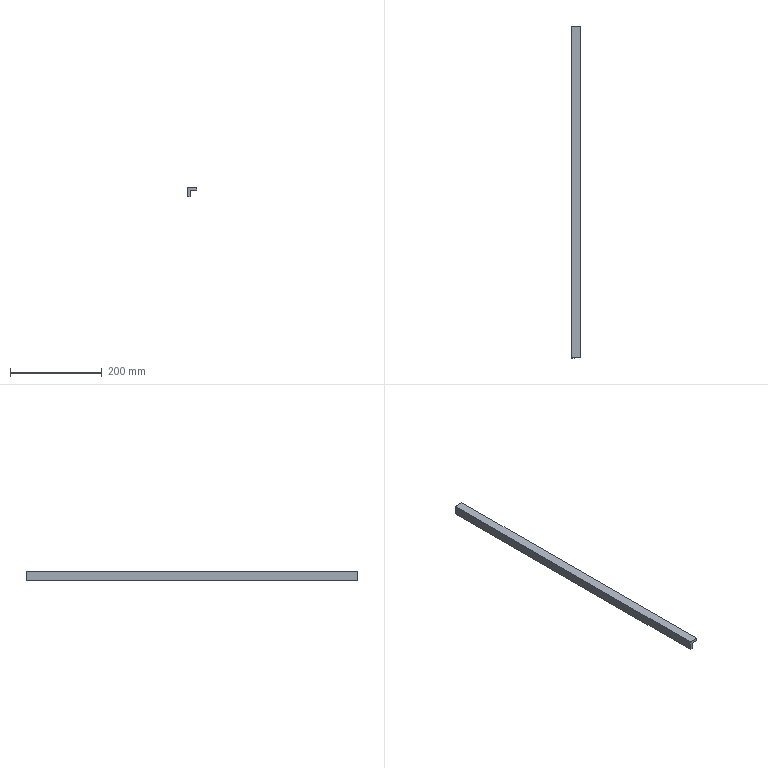Part | NX | 1 solid | 8 faces | box 20 x 724.234 x 20 mm | volume 147744 mm3 | plane 8
STEP:
#1=CARTESIAN_POINT('',(0.,-324.234,0.));
#2=VERTEX_POINT('',#1);
#3=CARTESIAN_POINT('',(20.,-324.234,0.));
#4=VERTEX_POINT('',#3);
#5=CARTESIAN_POINT('',(-266.252,-324.234,0.));
#6=DIRECTION('',(1.,0.,0.));
#7=VECTOR('',#6,1.);
#8=LINE('',#5,#7);
#9=EDGE_CURVE('',#2,#4,#8,.T.);
#10=ORIENTED_EDGE('',*,*,#9,.T.);
#11=CARTESIAN_POINT('',(20.,400.,0.));
#12=VERTEX_POINT('',#11);
#13=CARTESIAN_POINT('',(20.,400.,0.));
#14=DIRECTION('',(0.,-1.,0.));
#15=VECTOR('',#14,1.);
#16=LINE('',#13,#15);
#17=EDGE_CURVE('',#12,#4,#16,.T.);
#18=ORIENTED_EDGE('',*,*,#17,.F.);
#19=CARTESIAN_POINT('',(0.,400.,0.));
#20=VERTEX_POINT('',#19);
#21=CARTESIAN_POINT('',(20.,400.,0.));
#22=DIRECTION('',(1.,0.,0.));
#23=VECTOR('',#22,1.);
#24=LINE('',#21,#23);
#25=EDGE_CURVE('',#20,#12,#24,.T.);
#26=ORIENTED_EDGE('',*,*,#25,.F.);
#27=CARTESIAN_POINT('',(0.,400.,0.));
#28=DIRECTION('',(0.,-1.,0.));
#29=VECTOR('',#28,1.);
#30=LINE('',#27,#29);
#31=EDGE_CURVE('',#20,#2,#30,.T.);
#32=ORIENTED_EDGE('',*,*,#31,.T.);
#33=EDGE_LOOP('',(#10,#18,#26,#32));
#34=FACE_OUTER_BOUND('',#33,.T.);
#35=CARTESIAN_POINT('',(20.,400.,0.));
#36=DIRECTION('',(0.,0.,-1.));
#37=DIRECTION('',(-1.,0.,0.));
#38=AXIS2_PLACEMENT_3D('',#35,#36,#37);
#39=PLANE('',#38);
#40=ADVANCED_FACE('',(#34),#39,.F.);
#41=CARTESIAN_POINT('',(20.,-324.234,-6.));
#42=VERTEX_POINT('',#41);
#43=CARTESIAN_POINT('',(20.,-324.234,-229.311));
#44=DIRECTION('',(0.,0.,-1.));
#45=VECTOR('',#44,1.);
#46=LINE('',#43,#45);
#47=EDGE_CURVE('',#4,#42,#46,.T.);
#48=ORIENTED_EDGE('',*,*,#47,.T.);
#49=CARTESIAN_POINT('',(20.,400.,-6.));
#50=VERTEX_POINT('',#49);
#51=CARTESIAN_POINT('',(20.,400.,-6.));
#52=DIRECTION('',(0.,-1.,0.));
#53=VECTOR('',#52,1.);
#54=LINE('',#51,#53);
#55=EDGE_CURVE('',#50,#42,#54,.T.);
#56=ORIENTED_EDGE('',*,*,#55,.F.);
#57=CARTESIAN_POINT('',(20.,400.,-6.));
#58=DIRECTION('',(0.,0.,-1.));
#59=VECTOR('',#58,1.);
#60=LINE('',#57,#59);
#61=EDGE_CURVE('',#12,#50,#60,.T.);
#62=ORIENTED_EDGE('',*,*,#61,.F.);
#63=ORIENTED_EDGE('',*,*,#17,.T.);
#64=EDGE_LOOP('',(#48,#56,#62,#63));
#65=FACE_OUTER_BOUND('',#64,.T.);
#66=CARTESIAN_POINT('',(20.,400.,-6.));
#67=DIRECTION('',(-1.,0.,0.));
#68=DIRECTION('',(0.,0.,1.));
#69=AXIS2_PLACEMENT_3D('',#66,#67,#68);
#70=PLANE('',#69);
#71=ADVANCED_FACE('',(#65),#70,.F.);
#72=CARTESIAN_POINT('',(6.,-324.234,-6.));
#73=VERTEX_POINT('',#72);
#74=CARTESIAN_POINT('',(-266.252,-324.234,-6.));
#75=DIRECTION('',(-1.,0.,0.));
#76=VECTOR('',#75,1.);
#77=LINE('',#74,#76);
#78=EDGE_CURVE('',#42,#73,#77,.T.);
#79=ORIENTED_EDGE('',*,*,#78,.T.);
#80=CARTESIAN_POINT('',(6.,400.,-6.));
#81=VERTEX_POINT('',#80);
#82=CARTESIAN_POINT('',(6.,400.,-6.));
#83=DIRECTION('',(0.,-1.,0.));
#84=VECTOR('',#83,1.);
#85=LINE('',#82,#84);
#86=EDGE_CURVE('',#81,#73,#85,.T.);
#87=ORIENTED_EDGE('',*,*,#86,.F.);
#88=CARTESIAN_POINT('',(6.,400.,-6.));
#89=DIRECTION('',(-1.,0.,0.));
#90=VECTOR('',#89,1.);
#91=LINE('',#88,#90);
#92=EDGE_CURVE('',#50,#81,#91,.T.);
#93=ORIENTED_EDGE('',*,*,#92,.F.);
#94=ORIENTED_EDGE('',*,*,#55,.T.);
#95=EDGE_LOOP('',(#79,#87,#93,#94));
#96=FACE_OUTER_BOUND('',#95,.T.);
#97=CARTESIAN_POINT('',(6.,400.,-6.));
#98=DIRECTION('',(0.,0.,1.));
#99=DIRECTION('',(1.,0.,0.));
#100=AXIS2_PLACEMENT_3D('',#97,#98,#99);
#101=PLANE('',#100);
#102=ADVANCED_FACE('',(#96),#101,.F.);
#103=CARTESIAN_POINT('',(6.,-324.234,-20.));
#104=VERTEX_POINT('',#103);
#105=CARTESIAN_POINT('',(6.,-324.234,-229.311));
#106=DIRECTION('',(0.,0.,-1.));
#107=VECTOR('',#106,1.);
#108=LINE('',#105,#107);
#109=EDGE_CURVE('',#73,#104,#108,.T.);
#110=ORIENTED_EDGE('',*,*,#109,.T.);
#111=CARTESIAN_POINT('',(6.,400.,-20.));
#112=VERTEX_POINT('',#111);
#113=CARTESIAN_POINT('',(6.,400.,-20.));
#114=DIRECTION('',(0.,-1.,0.));
#115=VECTOR('',#114,1.);
#116=LINE('',#113,#115);
#117=EDGE_CURVE('',#112,#104,#116,.T.);
#118=ORIENTED_EDGE('',*,*,#117,.F.);
#119=CARTESIAN_POINT('',(6.,400.,-20.));
#120=DIRECTION('',(0.,0.,-1.));
#121=VECTOR('',#120,1.);
#122=LINE('',#119,#121);
#123=EDGE_CURVE('',#81,#112,#122,.T.);
#124=ORIENTED_EDGE('',*,*,#123,.F.);
#125=ORIENTED_EDGE('',*,*,#86,.T.);
#126=EDGE_LOOP('',(#110,#118,#124,#125));
#127=FACE_OUTER_BOUND('',#126,.T.);
#128=CARTESIAN_POINT('',(6.,400.,-20.));
#129=DIRECTION('',(-1.,0.,0.));
#130=DIRECTION('',(0.,0.,1.));
#131=AXIS2_PLACEMENT_3D('',#128,#129,#130);
#132=PLANE('',#131);
#133=ADVANCED_FACE('',(#127),#132,.F.);
#134=CARTESIAN_POINT('',(0.,-324.234,-20.));
#135=VERTEX_POINT('',#134);
#136=CARTESIAN_POINT('',(-266.252,-324.234,-20.));
#137=DIRECTION('',(-1.,0.,0.));
#138=VECTOR('',#137,1.);
#139=LINE('',#136,#138);
#140=EDGE_CURVE('',#104,#135,#139,.T.);
#141=ORIENTED_EDGE('',*,*,#140,.T.);
#142=CARTESIAN_POINT('',(0.,400.,-20.));
#143=VERTEX_POINT('',#142);
#144=CARTESIAN_POINT('',(0.,400.,-20.));
#145=DIRECTION('',(0.,-1.,0.));
#146=VECTOR('',#145,1.);
#147=LINE('',#144,#146);
#148=EDGE_CURVE('',#143,#135,#147,.T.);
#149=ORIENTED_EDGE('',*,*,#148,.F.);
#150=CARTESIAN_POINT('',(0.,400.,-20.));
#151=DIRECTION('',(-1.,0.,0.));
#152=VECTOR('',#151,1.);
#153=LINE('',#150,#152);
#154=EDGE_CURVE('',#112,#143,#153,.T.);
#155=ORIENTED_EDGE('',*,*,#154,.F.);
#156=ORIENTED_EDGE('',*,*,#117,.T.);
#157=EDGE_LOOP('',(#141,#149,#155,#156));
#158=FACE_OUTER_BOUND('',#157,.T.);
#159=CARTESIAN_POINT('',(0.,400.,-20.));
#160=DIRECTION('',(0.,0.,1.));
#161=DIRECTION('',(1.,0.,0.));
#162=AXIS2_PLACEMENT_3D('',#159,#160,#161);
#163=PLANE('',#162);
#164=ADVANCED_FACE('',(#158),#163,.F.);
#165=CARTESIAN_POINT('',(0.,-324.234,-229.311));
#166=DIRECTION('',(0.,0.,1.));
#167=VECTOR('',#166,1.);
#168=LINE('',#165,#167);
#169=EDGE_CURVE('',#135,#2,#168,.T.);
#170=ORIENTED_EDGE('',*,*,#169,.T.);
#171=ORIENTED_EDGE('',*,*,#31,.F.);
#172=CARTESIAN_POINT('',(0.,400.,0.));
#173=DIRECTION('',(0.,0.,1.));
#174=VECTOR('',#173,1.);
#175=LINE('',#172,#174);
#176=EDGE_CURVE('',#143,#20,#175,.T.);
#177=ORIENTED_EDGE('',*,*,#176,.F.);
#178=ORIENTED_EDGE('',*,*,#148,.T.);
#179=EDGE_LOOP('',(#170,#171,#177,#178));
#180=FACE_OUTER_BOUND('',#179,.T.);
#181=CARTESIAN_POINT('',(0.,400.,0.));
#182=DIRECTION('',(1.,0.,0.));
#183=DIRECTION('',(0.,0.,-1.));
#184=AXIS2_PLACEMENT_3D('',#181,#182,#183);
#185=PLANE('',#184);
#186=ADVANCED_FACE('',(#180),#185,.F.);
#187=ORIENTED_EDGE('',*,*,#25,.T.);
#188=ORIENTED_EDGE('',*,*,#61,.T.);
#189=ORIENTED_EDGE('',*,*,#92,.T.);
#190=ORIENTED_EDGE('',*,*,#123,.T.);
#191=ORIENTED_EDGE('',*,*,#154,.T.);
#192=ORIENTED_EDGE('',*,*,#176,.T.);
#193=EDGE_LOOP('',(#187,#188,#189,#190,#191,#192));
#194=FACE_OUTER_BOUND('',#193,.T.);
#195=CARTESIAN_POINT('',(0.,400.,0.));
#196=DIRECTION('',(0.,-1.,0.));
#197=DIRECTION('',(0.,0.,-1.));
#198=AXIS2_PLACEMENT_3D('',#195,#196,#197);
#199=PLANE('',#198);
#200=ADVANCED_FACE('',(#194),#199,.F.);
#201=ORIENTED_EDGE('',*,*,#9,.F.);
#202=ORIENTED_EDGE('',*,*,#169,.F.);
#203=ORIENTED_EDGE('',*,*,#140,.F.);
#204=ORIENTED_EDGE('',*,*,#109,.F.);
#205=ORIENTED_EDGE('',*,*,#78,.F.);
#206=ORIENTED_EDGE('',*,*,#47,.F.);
#207=EDGE_LOOP('',(#201,#202,#203,#204,#205,#206));
#208=FACE_OUTER_BOUND('',#207,.T.);
#209=CARTESIAN_POINT('',(-266.252,-324.234,-229.311));
#210=DIRECTION('',(0.,-1.,0.));
#211=DIRECTION('',(-0.866,0.,-0.5));
#212=AXIS2_PLACEMENT_3D('',#209,#210,#211);
#213=PLANE('',#212);
#214=ADVANCED_FACE('',(#208),#213,.T.);
#215=CLOSED_SHELL('',(#40,#71,#102,#133,#164,#186,#200,#214));
#216=MANIFOLD_SOLID_BREP('',#215);
#217=(LENGTH_UNIT()NAMED_UNIT(*)SI_UNIT(.MILLI.,.METRE.));
#218=UNCERTAINTY_MEASURE_WITH_UNIT(LENGTH_MEASURE(0.00002),#217,'','');
#219=(NAMED_UNIT(*)PLANE_ANGLE_UNIT()SI_UNIT($,.RADIAN.));
#220=PLANE_ANGLE_MEASURE_WITH_UNIT(PLANE_ANGLE_MEASURE(0.01745),#219);
#221=DIMENSIONAL_EXPONENTS(0.,0.,0.,0.,0.,0.,0.);
#222=(CONVERSION_BASED_UNIT('DEGREE',#220)NAMED_UNIT(#221)PLANE_ANGLE_UNIT());
#223=(NAMED_UNIT(*)SI_UNIT($,.STERADIAN.)SOLID_ANGLE_UNIT());
#224=(GEOMETRIC_REPRESENTATION_CONTEXT(3)GLOBAL_UNCERTAINTY_ASSIGNED_CONTEXT((#218))GLOBAL_UNIT_ASSIGNED_CONTEXT((#217,#222,#223))REPRESENTATION_CONTEXT('',''));
#225=ADVANCED_BREP_SHAPE_REPRESENTATION('',(#216),#224);